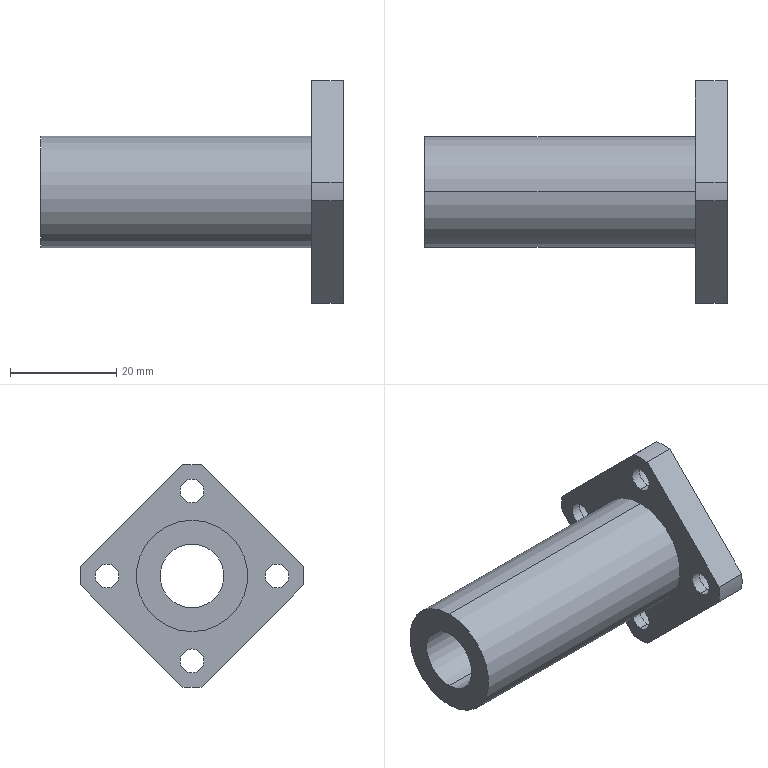Part | SolidWorks | features HoleWzd 2, ICE 2, CirPattern 1, Extrusion 1 | 1 solid | 36 faces | box 57 x 42 x 42 mm | volume 16451 mm3 | cylinder 25 | plane 11 | commonest cylinder face diameters 4.5 x8 7.5 x8 42 x5 12 x2 21 x2
STEP:
#1=CARTESIAN_POINT('',(22.5,0.,-13.75));
#2=VERTEX_POINT('',#1);
#3=CARTESIAN_POINT('',(22.5,0.,-18.25));
#4=VERTEX_POINT('',#3);
#5=CARTESIAN_POINT('',(22.5,0.,-16.));
#6=DIRECTION('',(1.,0.,0.));
#7=DIRECTION('',(0.,0.,-1.));
#8=AXIS2_PLACEMENT_3D('',#5,#6,#7);
#9=CIRCLE('',#8,2.25);
#10=EDGE_CURVE('',#2,#4,#9,.T.);
#11=ORIENTED_EDGE('',*,*,#10,.F.);
#12=CARTESIAN_POINT('',(24.4,0.,-13.75));
#13=VERTEX_POINT('',#12);
#14=CARTESIAN_POINT('',(24.4,0.,-13.75));
#15=DIRECTION('',(1.,0.,0.));
#16=VECTOR('',#15,1000.);
#17=LINE('',#14,#16);
#18=EDGE_CURVE('',#2,#13,#17,.T.);
#19=ORIENTED_EDGE('',*,*,#18,.T.);
#20=CARTESIAN_POINT('',(24.4,0.,-18.25));
#21=VERTEX_POINT('',#20);
#22=CARTESIAN_POINT('',(24.4,0.,-16.));
#23=DIRECTION('',(1.,0.,0.));
#24=DIRECTION('',(0.,0.,-1.));
#25=AXIS2_PLACEMENT_3D('',#22,#23,#24);
#26=CIRCLE('',#25,2.25);
#27=EDGE_CURVE('',#13,#21,#26,.T.);
#28=ORIENTED_EDGE('',*,*,#27,.T.);
#29=CARTESIAN_POINT('',(24.4,0.,-18.25));
#30=DIRECTION('',(1.,0.,0.));
#31=VECTOR('',#30,1000.);
#32=LINE('',#29,#31);
#33=EDGE_CURVE('',#4,#21,#32,.T.);
#34=ORIENTED_EDGE('',*,*,#33,.F.);
#35=EDGE_LOOP('',(#11,#19,#28,#34));
#36=FACE_OUTER_BOUND('',#35,.T.);
#37=CARTESIAN_POINT('',(24.4,0.,-16.));
#38=DIRECTION('',(1.,0.,0.));
#39=DIRECTION('',(0.,0.,-1.));
#40=AXIS2_PLACEMENT_3D('',#37,#38,#39);
#41=CYLINDRICAL_SURFACE('',#40,2.25);
#42=ADVANCED_FACE('',(#36),#41,.F.);
#43=CARTESIAN_POINT('',(22.5,-16.,2.25));
#44=VERTEX_POINT('',#43);
#45=CARTESIAN_POINT('',(22.5,-16.,-2.25));
#46=VERTEX_POINT('',#45);
#47=CARTESIAN_POINT('',(22.5,-16.,0.));
#48=DIRECTION('',(1.,0.,0.));
#49=DIRECTION('',(0.,0.,-1.));
#50=AXIS2_PLACEMENT_3D('',#47,#48,#49);
#51=CIRCLE('',#50,2.25);
#52=EDGE_CURVE('',#44,#46,#51,.T.);
#53=ORIENTED_EDGE('',*,*,#52,.F.);
#54=CARTESIAN_POINT('',(24.4,-16.,2.25));
#55=VERTEX_POINT('',#54);
#56=CARTESIAN_POINT('',(24.4,-16.,2.25));
#57=DIRECTION('',(1.,0.,0.));
#58=VECTOR('',#57,1000.);
#59=LINE('',#56,#58);
#60=EDGE_CURVE('',#44,#55,#59,.T.);
#61=ORIENTED_EDGE('',*,*,#60,.T.);
#62=CARTESIAN_POINT('',(24.4,-16.,-2.25));
#63=VERTEX_POINT('',#62);
#64=CARTESIAN_POINT('',(24.4,-16.,0.));
#65=DIRECTION('',(1.,0.,0.));
#66=DIRECTION('',(0.,0.,-1.));
#67=AXIS2_PLACEMENT_3D('',#64,#65,#66);
#68=CIRCLE('',#67,2.25);
#69=EDGE_CURVE('',#55,#63,#68,.T.);
#70=ORIENTED_EDGE('',*,*,#69,.T.);
#71=CARTESIAN_POINT('',(24.4,-16.,-2.25));
#72=DIRECTION('',(1.,0.,0.));
#73=VECTOR('',#72,1000.);
#74=LINE('',#71,#73);
#75=EDGE_CURVE('',#46,#63,#74,.T.);
#76=ORIENTED_EDGE('',*,*,#75,.F.);
#77=EDGE_LOOP('',(#53,#61,#70,#76));
#78=FACE_OUTER_BOUND('',#77,.T.);
#79=CARTESIAN_POINT('',(24.4,-16.,0.));
#80=DIRECTION('',(1.,0.,0.));
#81=DIRECTION('',(0.,0.,-1.));
#82=AXIS2_PLACEMENT_3D('',#79,#80,#81);
#83=CYLINDRICAL_SURFACE('',#82,2.25);
#84=ADVANCED_FACE('',(#78),#83,.F.);
#85=CARTESIAN_POINT('',(22.5,0.,18.25));
#86=VERTEX_POINT('',#85);
#87=CARTESIAN_POINT('',(22.5,0.,13.75));
#88=VERTEX_POINT('',#87);
#89=CARTESIAN_POINT('',(22.5,0.,16.));
#90=DIRECTION('',(1.,0.,0.));
#91=DIRECTION('',(0.,0.,-1.));
#92=AXIS2_PLACEMENT_3D('',#89,#90,#91);
#93=CIRCLE('',#92,2.25);
#94=EDGE_CURVE('',#86,#88,#93,.T.);
#95=ORIENTED_EDGE('',*,*,#94,.F.);
#96=CARTESIAN_POINT('',(24.4,0.,18.25));
#97=VERTEX_POINT('',#96);
#98=CARTESIAN_POINT('',(24.4,0.,18.25));
#99=DIRECTION('',(1.,0.,0.));
#100=VECTOR('',#99,1000.);
#101=LINE('',#98,#100);
#102=EDGE_CURVE('',#86,#97,#101,.T.);
#103=ORIENTED_EDGE('',*,*,#102,.T.);
#104=CARTESIAN_POINT('',(24.4,0.,13.75));
#105=VERTEX_POINT('',#104);
#106=CARTESIAN_POINT('',(24.4,0.,16.));
#107=DIRECTION('',(1.,0.,0.));
#108=DIRECTION('',(0.,0.,-1.));
#109=AXIS2_PLACEMENT_3D('',#106,#107,#108);
#110=CIRCLE('',#109,2.25);
#111=EDGE_CURVE('',#97,#105,#110,.T.);
#112=ORIENTED_EDGE('',*,*,#111,.T.);
#113=CARTESIAN_POINT('',(24.4,0.,13.75));
#114=DIRECTION('',(1.,0.,0.));
#115=VECTOR('',#114,1000.);
#116=LINE('',#113,#115);
#117=EDGE_CURVE('',#88,#105,#116,.T.);
#118=ORIENTED_EDGE('',*,*,#117,.F.);
#119=EDGE_LOOP('',(#95,#103,#112,#118));
#120=FACE_OUTER_BOUND('',#119,.T.);
#121=CARTESIAN_POINT('',(24.4,0.,16.));
#122=DIRECTION('',(1.,0.,0.));
#123=DIRECTION('',(0.,0.,-1.));
#124=AXIS2_PLACEMENT_3D('',#121,#122,#123);
#125=CYLINDRICAL_SURFACE('',#124,2.25);
#126=ADVANCED_FACE('',(#120),#125,.F.);
#127=CARTESIAN_POINT('',(24.4,0.,-12.25));
#128=VERTEX_POINT('',#127);
#129=CARTESIAN_POINT('',(24.4,0.,-19.75));
#130=VERTEX_POINT('',#129);
#131=CARTESIAN_POINT('',(24.4,0.,-16.));
#132=DIRECTION('',(1.,0.,0.));
#133=DIRECTION('',(0.,0.,-1.));
#134=AXIS2_PLACEMENT_3D('',#131,#132,#133);
#135=CIRCLE('',#134,3.75);
#136=EDGE_CURVE('',#128,#130,#135,.T.);
#137=ORIENTED_EDGE('',*,*,#136,.F.);
#138=CARTESIAN_POINT('',(28.5,0.,-12.25));
#139=VERTEX_POINT('',#138);
#140=CARTESIAN_POINT('',(28.5,0.,-12.25));
#141=DIRECTION('',(1.,0.,0.));
#142=VECTOR('',#141,1000.);
#143=LINE('',#140,#142);
#144=EDGE_CURVE('',#128,#139,#143,.T.);
#145=ORIENTED_EDGE('',*,*,#144,.T.);
#146=CARTESIAN_POINT('',(28.5,0.,-19.75));
#147=VERTEX_POINT('',#146);
#148=CARTESIAN_POINT('',(28.5,0.,-16.));
#149=DIRECTION('',(1.,0.,0.));
#150=DIRECTION('',(0.,0.,-1.));
#151=AXIS2_PLACEMENT_3D('',#148,#149,#150);
#152=CIRCLE('',#151,3.75);
#153=EDGE_CURVE('',#139,#147,#152,.T.);
#154=ORIENTED_EDGE('',*,*,#153,.T.);
#155=CARTESIAN_POINT('',(28.5,0.,-19.75));
#156=DIRECTION('',(1.,0.,0.));
#157=VECTOR('',#156,1000.);
#158=LINE('',#155,#157);
#159=EDGE_CURVE('',#130,#147,#158,.T.);
#160=ORIENTED_EDGE('',*,*,#159,.F.);
#161=EDGE_LOOP('',(#137,#145,#154,#160));
#162=FACE_OUTER_BOUND('',#161,.T.);
#163=CARTESIAN_POINT('',(28.5,0.,-16.));
#164=DIRECTION('',(1.,0.,0.));
#165=DIRECTION('',(0.,0.,-1.));
#166=AXIS2_PLACEMENT_3D('',#163,#164,#165);
#167=CYLINDRICAL_SURFACE('',#166,3.75);
#168=ADVANCED_FACE('',(#162),#167,.F.);
#169=CARTESIAN_POINT('',(24.4,-16.,3.75));
#170=VERTEX_POINT('',#169);
#171=CARTESIAN_POINT('',(24.4,-16.,-3.75));
#172=VERTEX_POINT('',#171);
#173=CARTESIAN_POINT('',(24.4,-16.,0.));
#174=DIRECTION('',(1.,0.,0.));
#175=DIRECTION('',(0.,0.,-1.));
#176=AXIS2_PLACEMENT_3D('',#173,#174,#175);
#177=CIRCLE('',#176,3.75);
#178=EDGE_CURVE('',#170,#172,#177,.T.);
#179=ORIENTED_EDGE('',*,*,#178,.F.);
#180=CARTESIAN_POINT('',(28.5,-16.,3.75));
#181=VERTEX_POINT('',#180);
#182=CARTESIAN_POINT('',(28.5,-16.,3.75));
#183=DIRECTION('',(1.,0.,0.));
#184=VECTOR('',#183,1000.);
#185=LINE('',#182,#184);
#186=EDGE_CURVE('',#170,#181,#185,.T.);
#187=ORIENTED_EDGE('',*,*,#186,.T.);
#188=CARTESIAN_POINT('',(28.5,-16.,-3.75));
#189=VERTEX_POINT('',#188);
#190=CARTESIAN_POINT('',(28.5,-16.,0.));
#191=DIRECTION('',(1.,0.,0.));
#192=DIRECTION('',(0.,0.,-1.));
#193=AXIS2_PLACEMENT_3D('',#190,#191,#192);
#194=CIRCLE('',#193,3.75);
#195=EDGE_CURVE('',#181,#189,#194,.T.);
#196=ORIENTED_EDGE('',*,*,#195,.T.);
#197=CARTESIAN_POINT('',(28.5,-16.,-3.75));
#198=DIRECTION('',(1.,0.,0.));
#199=VECTOR('',#198,1000.);
#200=LINE('',#197,#199);
#201=EDGE_CURVE('',#172,#189,#200,.T.);
#202=ORIENTED_EDGE('',*,*,#201,.F.);
#203=EDGE_LOOP('',(#179,#187,#196,#202));
#204=FACE_OUTER_BOUND('',#203,.T.);
#205=CARTESIAN_POINT('',(28.5,-16.,0.));
#206=DIRECTION('',(1.,0.,0.));
#207=DIRECTION('',(0.,0.,-1.));
#208=AXIS2_PLACEMENT_3D('',#205,#206,#207);
#209=CYLINDRICAL_SURFACE('',#208,3.75);
#210=ADVANCED_FACE('',(#204),#209,.F.);
#211=CARTESIAN_POINT('',(24.4,0.,19.75));
#212=VERTEX_POINT('',#211);
#213=CARTESIAN_POINT('',(24.4,0.,12.25));
#214=VERTEX_POINT('',#213);
#215=CARTESIAN_POINT('',(24.4,0.,16.));
#216=DIRECTION('',(1.,0.,0.));
#217=DIRECTION('',(0.,0.,-1.));
#218=AXIS2_PLACEMENT_3D('',#215,#216,#217);
#219=CIRCLE('',#218,3.75);
#220=EDGE_CURVE('',#212,#214,#219,.T.);
#221=ORIENTED_EDGE('',*,*,#220,.F.);
#222=CARTESIAN_POINT('',(28.5,0.,19.75));
#223=VERTEX_POINT('',#222);
#224=CARTESIAN_POINT('',(28.5,0.,19.75));
#225=DIRECTION('',(1.,0.,0.));
#226=VECTOR('',#225,1000.);
#227=LINE('',#224,#226);
#228=EDGE_CURVE('',#212,#223,#227,.T.);
#229=ORIENTED_EDGE('',*,*,#228,.T.);
#230=CARTESIAN_POINT('',(28.5,0.,12.25));
#231=VERTEX_POINT('',#230);
#232=CARTESIAN_POINT('',(28.5,0.,16.));
#233=DIRECTION('',(1.,0.,0.));
#234=DIRECTION('',(0.,0.,-1.));
#235=AXIS2_PLACEMENT_3D('',#232,#233,#234);
#236=CIRCLE('',#235,3.75);
#237=EDGE_CURVE('',#223,#231,#236,.T.);
#238=ORIENTED_EDGE('',*,*,#237,.T.);
#239=CARTESIAN_POINT('',(28.5,0.,12.25));
#240=DIRECTION('',(1.,0.,0.));
#241=VECTOR('',#240,1000.);
#242=LINE('',#239,#241);
#243=EDGE_CURVE('',#214,#231,#242,.T.);
#244=ORIENTED_EDGE('',*,*,#243,.F.);
#245=EDGE_LOOP('',(#221,#229,#238,#244));
#246=FACE_OUTER_BOUND('',#245,.T.);
#247=CARTESIAN_POINT('',(28.5,0.,16.));
#248=DIRECTION('',(1.,0.,0.));
#249=DIRECTION('',(0.,0.,-1.));
#250=AXIS2_PLACEMENT_3D('',#247,#248,#249);
#251=CYLINDRICAL_SURFACE('',#250,3.75);
#252=ADVANCED_FACE('',(#246),#251,.F.);
#253=CARTESIAN_POINT('',(22.5,16.,2.25));
#254=VERTEX_POINT('',#253);
#255=CARTESIAN_POINT('',(22.5,16.,-2.25));
#256=VERTEX_POINT('',#255);
#257=CARTESIAN_POINT('',(22.5,16.,0.));
#258=DIRECTION('',(1.,0.,0.));
#259=DIRECTION('',(0.,0.,-1.));
#260=AXIS2_PLACEMENT_3D('',#257,#258,#259);
#261=CIRCLE('',#260,2.25);
#262=EDGE_CURVE('',#254,#256,#261,.T.);
#263=ORIENTED_EDGE('',*,*,#262,.F.);
#264=CARTESIAN_POINT('',(24.4,16.,2.25));
#265=VERTEX_POINT('',#264);
#266=CARTESIAN_POINT('',(24.4,16.,2.25));
#267=DIRECTION('',(1.,0.,0.));
#268=VECTOR('',#267,1000.);
#269=LINE('',#266,#268);
#270=EDGE_CURVE('',#254,#265,#269,.T.);
#271=ORIENTED_EDGE('',*,*,#270,.T.);
#272=CARTESIAN_POINT('',(24.4,16.,-2.25));
#273=VERTEX_POINT('',#272);
#274=CARTESIAN_POINT('',(24.4,16.,0.));
#275=DIRECTION('',(1.,0.,0.));
#276=DIRECTION('',(0.,0.,-1.));
#277=AXIS2_PLACEMENT_3D('',#274,#275,#276);
#278=CIRCLE('',#277,2.25);
#279=EDGE_CURVE('',#265,#273,#278,.T.);
#280=ORIENTED_EDGE('',*,*,#279,.T.);
#281=CARTESIAN_POINT('',(24.4,16.,-2.25));
#282=DIRECTION('',(1.,0.,0.));
#283=VECTOR('',#282,1000.);
#284=LINE('',#281,#283);
#285=EDGE_CURVE('',#256,#273,#284,.T.);
#286=ORIENTED_EDGE('',*,*,#285,.F.);
#287=EDGE_LOOP('',(#263,#271,#280,#286));
#288=FACE_OUTER_BOUND('',#287,.T.);
#289=CARTESIAN_POINT('',(24.4,16.,0.));
#290=DIRECTION('',(1.,0.,0.));
#291=DIRECTION('',(0.,0.,-1.));
#292=AXIS2_PLACEMENT_3D('',#289,#290,#291);
#293=CYLINDRICAL_SURFACE('',#292,2.25);
#294=ADVANCED_FACE('',(#288),#293,.F.);
#295=CARTESIAN_POINT('',(24.4,16.,3.75));
#296=VERTEX_POINT('',#295);
#297=CARTESIAN_POINT('',(24.4,16.,-3.75));
#298=VERTEX_POINT('',#297);
#299=CARTESIAN_POINT('',(24.4,16.,0.));
#300=DIRECTION('',(1.,0.,0.));
#301=DIRECTION('',(0.,0.,-1.));
#302=AXIS2_PLACEMENT_3D('',#299,#300,#301);
#303=CIRCLE('',#302,3.75);
#304=EDGE_CURVE('',#296,#298,#303,.T.);
#305=ORIENTED_EDGE('',*,*,#304,.F.);
#306=CARTESIAN_POINT('',(28.5,16.,3.75));
#307=VERTEX_POINT('',#306);
#308=CARTESIAN_POINT('',(28.5,16.,3.75));
#309=DIRECTION('',(1.,0.,0.));
#310=VECTOR('',#309,1000.);
#311=LINE('',#308,#310);
#312=EDGE_CURVE('',#296,#307,#311,.T.);
#313=ORIENTED_EDGE('',*,*,#312,.T.);
#314=CARTESIAN_POINT('',(28.5,16.,-3.75));
#315=VERTEX_POINT('',#314);
#316=CARTESIAN_POINT('',(28.5,16.,0.));
#317=DIRECTION('',(1.,0.,0.));
#318=DIRECTION('',(0.,0.,-1.));
#319=AXIS2_PLACEMENT_3D('',#316,#317,#318);
#320=CIRCLE('',#319,3.75);
#321=EDGE_CURVE('',#307,#315,#320,.T.);
#322=ORIENTED_EDGE('',*,*,#321,.T.);
#323=CARTESIAN_POINT('',(28.5,16.,-3.75));
#324=DIRECTION('',(1.,0.,0.));
#325=VECTOR('',#324,1000.);
#326=LINE('',#323,#325);
#327=EDGE_CURVE('',#298,#315,#326,.T.);
#328=ORIENTED_EDGE('',*,*,#327,.F.);
#329=EDGE_LOOP('',(#305,#313,#322,#328));
#330=FACE_OUTER_BOUND('',#329,.T.);
#331=CARTESIAN_POINT('',(28.5,16.,0.));
#332=DIRECTION('',(1.,0.,0.));
#333=DIRECTION('',(0.,0.,-1.));
#334=AXIS2_PLACEMENT_3D('',#331,#332,#333);
#335=CYLINDRICAL_SURFACE('',#334,3.75);
#336=ADVANCED_FACE('',(#330),#335,.F.);
#337=CARTESIAN_POINT('',(22.5,-1.696,-20.931));
#338=VERTEX_POINT('',#337);
#339=CARTESIAN_POINT('',(22.5,0.,-21.));
#340=VERTEX_POINT('',#339);
#341=CARTESIAN_POINT('',(22.5,0.,0.));
#342=DIRECTION('',(1.,0.,0.));
#343=DIRECTION('',(0.,0.,-1.));
#344=AXIS2_PLACEMENT_3D('',#341,#342,#343);
#345=CIRCLE('',#344,21.);
#346=EDGE_CURVE('',#338,#340,#345,.T.);
#347=ORIENTED_EDGE('',*,*,#346,.T.);
#348=CARTESIAN_POINT('',(28.5,0.,-21.));
#349=VERTEX_POINT('',#348);
#350=CARTESIAN_POINT('',(22.5,0.,-21.));
#351=DIRECTION('',(1.,0.,0.));
#352=VECTOR('',#351,1000.);
#353=LINE('',#350,#352);
#354=EDGE_CURVE('',#340,#349,#353,.T.);
#355=ORIENTED_EDGE('',*,*,#354,.T.);
#356=CARTESIAN_POINT('',(28.5,-1.696,-20.931));
#357=VERTEX_POINT('',#356);
#358=CARTESIAN_POINT('',(28.5,0.,0.));
#359=DIRECTION('',(1.,0.,0.));
#360=DIRECTION('',(0.,0.,-1.));
#361=AXIS2_PLACEMENT_3D('',#358,#359,#360);
#362=CIRCLE('',#361,21.);
#363=EDGE_CURVE('',#357,#349,#362,.T.);
#364=ORIENTED_EDGE('',*,*,#363,.F.);
#365=CARTESIAN_POINT('',(22.5,-1.696,-20.931));
#366=DIRECTION('',(1.,0.,0.));
#367=VECTOR('',#366,1000.);
#368=LINE('',#365,#367);
#369=EDGE_CURVE('',#338,#357,#368,.T.);
#370=ORIENTED_EDGE('',*,*,#369,.F.);
#371=EDGE_LOOP('',(#347,#355,#364,#370));
#372=FACE_OUTER_BOUND('',#371,.T.);
#373=CARTESIAN_POINT('',(22.5,0.,0.));
#374=DIRECTION('',(1.,0.,0.));
#375=DIRECTION('',(0.,0.,-1.));
#376=AXIS2_PLACEMENT_3D('',#373,#374,#375);
#377=CYLINDRICAL_SURFACE('',#376,21.);
#378=ADVANCED_FACE('',(#372),#377,.T.);
#379=CARTESIAN_POINT('',(28.5,0.,6.));
#380=VERTEX_POINT('',#379);
#381=CARTESIAN_POINT('',(28.5,0.,-6.));
#382=VERTEX_POINT('',#381);
#383=CARTESIAN_POINT('',(28.5,0.,0.));
#384=DIRECTION('',(1.,0.,0.));
#385=DIRECTION('',(0.,0.,-1.));
#386=AXIS2_PLACEMENT_3D('',#383,#384,#385);
#387=CIRCLE('',#386,6.);
#388=EDGE_CURVE('',#380,#382,#387,.T.);
#389=ORIENTED_EDGE('',*,*,#388,.T.);
#390=CARTESIAN_POINT('',(-28.5,0.,-6.));
#391=VERTEX_POINT('',#390);
#392=CARTESIAN_POINT('',(28.5,0.,-6.));
#393=DIRECTION('',(-1.,0.,0.));
#394=VECTOR('',#393,1000.);
#395=LINE('',#392,#394);
#396=EDGE_CURVE('',#382,#391,#395,.T.);
#397=ORIENTED_EDGE('',*,*,#396,.T.);
#398=CARTESIAN_POINT('',(-28.5,0.,6.));
#399=VERTEX_POINT('',#398);
#400=CARTESIAN_POINT('',(-28.5,0.,0.));
#401=DIRECTION('',(1.,0.,0.));
#402=DIRECTION('',(0.,0.,-1.));
#403=AXIS2_PLACEMENT_3D('',#400,#401,#402);
#404=CIRCLE('',#403,6.);
#405=EDGE_CURVE('',#399,#391,#404,.T.);
#406=ORIENTED_EDGE('',*,*,#405,.F.);
#407=CARTESIAN_POINT('',(28.5,0.,6.));
#408=DIRECTION('',(-1.,0.,0.));
#409=VECTOR('',#408,1000.);
#410=LINE('',#407,#409);
#411=EDGE_CURVE('',#380,#399,#410,.T.);
#412=ORIENTED_EDGE('',*,*,#411,.F.);
#413=EDGE_LOOP('',(#389,#397,#406,#412));
#414=FACE_OUTER_BOUND('',#413,.T.);
#415=CARTESIAN_POINT('',(28.5,0.,0.));
#416=DIRECTION('',(-1.,0.,0.));
#417=DIRECTION('',(0.,0.,1.));
#418=AXIS2_PLACEMENT_3D('',#415,#416,#417);
#419=CYLINDRICAL_SURFACE('',#418,6.);
#420=ADVANCED_FACE('',(#414),#419,.F.);
#421=CARTESIAN_POINT('',(22.5,0.,-10.5));
#422=VERTEX_POINT('',#421);
#423=CARTESIAN_POINT('',(22.5,0.,10.5));
#424=VERTEX_POINT('',#423);
#425=CARTESIAN_POINT('',(22.5,0.,0.));
#426=DIRECTION('',(1.,0.,0.));
#427=DIRECTION('',(0.,0.,-1.));
#428=AXIS2_PLACEMENT_3D('',#425,#426,#427);
#429=CIRCLE('',#428,10.5);
#430=EDGE_CURVE('',#422,#424,#429,.T.);
#431=ORIENTED_EDGE('',*,*,#430,.F.);
#432=CARTESIAN_POINT('',(-28.5,0.,-10.5));
#433=VERTEX_POINT('',#432);
#434=CARTESIAN_POINT('',(28.5,0.,-10.5));
#435=DIRECTION('',(-1.,0.,0.));
#436=VECTOR('',#435,1000.);
#437=LINE('',#434,#436);
#438=EDGE_CURVE('',#422,#433,#437,.T.);
#439=ORIENTED_EDGE('',*,*,#438,.T.);
#440=CARTESIAN_POINT('',(-28.5,0.,10.5));
#441=VERTEX_POINT('',#440);
#442=CARTESIAN_POINT('',(-28.5,0.,0.));
#443=DIRECTION('',(1.,0.,0.));
#444=DIRECTION('',(0.,0.,-1.));
#445=AXIS2_PLACEMENT_3D('',#442,#443,#444);
#446=CIRCLE('',#445,10.5);
#447=EDGE_CURVE('',#433,#441,#446,.T.);
#448=ORIENTED_EDGE('',*,*,#447,.T.);
#449=CARTESIAN_POINT('',(28.5,0.,10.5));
#450=DIRECTION('',(-1.,0.,0.));
#451=VECTOR('',#450,1000.);
#452=LINE('',#449,#451);
#453=EDGE_CURVE('',#424,#441,#452,.T.);
#454=ORIENTED_EDGE('',*,*,#453,.F.);
#455=EDGE_LOOP('',(#431,#439,#448,#454));
#456=FACE_OUTER_BOUND('',#455,.T.);
#457=CARTESIAN_POINT('',(28.5,0.,0.));
#458=DIRECTION('',(-1.,0.,0.));
#459=DIRECTION('',(0.,0.,1.));
#460=AXIS2_PLACEMENT_3D('',#457,#458,#459);
#461=CYLINDRICAL_SURFACE('',#460,10.5);
#462=ADVANCED_FACE('',(#456),#461,.T.);
#463=CARTESIAN_POINT('',(28.5,-20.931,1.696));
#464=VERTEX_POINT('',#463);
#465=CARTESIAN_POINT('',(28.5,-20.931,-1.696));
#466=VERTEX_POINT('',#465);
#467=CARTESIAN_POINT('',(28.5,0.,0.));
#468=DIRECTION('',(1.,0.,0.));
#469=DIRECTION('',(0.,0.,-1.));
#470=AXIS2_PLACEMENT_3D('',#467,#468,#469);
#471=CIRCLE('',#470,21.);
#472=EDGE_CURVE('',#464,#466,#471,.T.);
#473=ORIENTED_EDGE('',*,*,#472,.F.);
#474=CARTESIAN_POINT('',(22.5,-20.931,1.696));
#475=VERTEX_POINT('',#474);
#476=CARTESIAN_POINT('',(22.5,-20.931,1.696));
#477=DIRECTION('',(1.,0.,0.));
#478=VECTOR('',#477,1000.);
#479=LINE('',#476,#478);
#480=EDGE_CURVE('',#475,#464,#479,.T.);
#481=ORIENTED_EDGE('',*,*,#480,.F.);
#482=CARTESIAN_POINT('',(22.5,-20.931,-1.696));
#483=VERTEX_POINT('',#482);
#484=CARTESIAN_POINT('',(22.5,0.,0.));
#485=DIRECTION('',(1.,0.,0.));
#486=DIRECTION('',(0.,0.,-1.));
#487=AXIS2_PLACEMENT_3D('',#484,#485,#486);
#488=CIRCLE('',#487,21.);
#489=EDGE_CURVE('',#475,#483,#488,.T.);
#490=ORIENTED_EDGE('',*,*,#489,.T.);
#491=CARTESIAN_POINT('',(22.5,-20.931,-1.696));
#492=DIRECTION('',(-1.,0.,0.));
#493=VECTOR('',#492,1000.);
#494=LINE('',#491,#493);
#495=EDGE_CURVE('',#466,#483,#494,.T.);
#496=ORIENTED_EDGE('',*,*,#495,.F.);
#497=EDGE_LOOP('',(#473,#481,#490,#496));
#498=FACE_OUTER_BOUND('',#497,.T.);
#499=CARTESIAN_POINT('',(22.5,0.,0.));
#500=DIRECTION('',(1.,0.,0.));
#501=DIRECTION('',(0.,0.,-1.));
#502=AXIS2_PLACEMENT_3D('',#499,#500,#501);
#503=CYLINDRICAL_SURFACE('',#502,21.);
#504=ADVANCED_FACE('',(#498),#503,.T.);
#505=CARTESIAN_POINT('',(22.5,1.696,20.931));
#506=VERTEX_POINT('',#505);
#507=CARTESIAN_POINT('',(22.5,-1.696,20.931));
#508=VERTEX_POINT('',#507);
#509=CARTESIAN_POINT('',(22.5,0.,0.));
#510=DIRECTION('',(1.,0.,0.));
#511=DIRECTION('',(0.,0.,-1.));
#512=AXIS2_PLACEMENT_3D('',#509,#510,#511);
#513=CIRCLE('',#512,21.);
#514=EDGE_CURVE('',#506,#508,#513,.T.);
#515=ORIENTED_EDGE('',*,*,#514,.T.);
#516=CARTESIAN_POINT('',(28.5,-1.696,20.931));
#517=VERTEX_POINT('',#516);
#518=CARTESIAN_POINT('',(22.5,-1.696,20.931));
#519=DIRECTION('',(-1.,0.,0.));
#520=VECTOR('',#519,1000.);
#521=LINE('',#518,#520);
#522=EDGE_CURVE('',#517,#508,#521,.T.);
#523=ORIENTED_EDGE('',*,*,#522,.F.);
#524=CARTESIAN_POINT('',(28.5,1.696,20.931));
#525=VERTEX_POINT('',#524);
#526=CARTESIAN_POINT('',(28.5,0.,0.));
#527=DIRECTION('',(1.,0.,0.));
#528=DIRECTION('',(0.,0.,-1.));
#529=AXIS2_PLACEMENT_3D('',#526,#527,#528);
#530=CIRCLE('',#529,21.);
#531=EDGE_CURVE('',#525,#517,#530,.T.);
#532=ORIENTED_EDGE('',*,*,#531,.F.);
#533=CARTESIAN_POINT('',(22.5,1.696,20.931));
#534=DIRECTION('',(1.,0.,0.));
#535=VECTOR('',#534,1000.);
#536=LINE('',#533,#535);
#537=EDGE_CURVE('',#506,#525,#536,.T.);
#538=ORIENTED_EDGE('',*,*,#537,.F.);
#539=EDGE_LOOP('',(#515,#523,#532,#538));
#540=FACE_OUTER_BOUND('',#539,.T.);
#541=CARTESIAN_POINT('',(22.5,0.,0.));
#542=DIRECTION('',(1.,0.,0.));
#543=DIRECTION('',(0.,0.,-1.));
#544=AXIS2_PLACEMENT_3D('',#541,#542,#543);
#545=CYLINDRICAL_SURFACE('',#544,21.);
#546=ADVANCED_FACE('',(#540),#545,.T.);
#547=CARTESIAN_POINT('',(22.5,20.931,-1.696));
#548=VERTEX_POINT('',#547);
#549=CARTESIAN_POINT('',(22.5,20.931,1.696));
#550=VERTEX_POINT('',#549);
#551=CARTESIAN_POINT('',(22.5,0.,0.));
#552=DIRECTION('',(1.,0.,0.));
#553=DIRECTION('',(0.,0.,-1.));
#554=AXIS2_PLACEMENT_3D('',#551,#552,#553);
#555=CIRCLE('',#554,21.);
#556=EDGE_CURVE('',#548,#550,#555,.T.);
#557=ORIENTED_EDGE('',*,*,#556,.T.);
#558=CARTESIAN_POINT('',(28.5,20.931,1.696));
#559=VERTEX_POINT('',#558);
#560=CARTESIAN_POINT('',(22.5,20.931,1.696));
#561=DIRECTION('',(-1.,0.,0.));
#562=VECTOR('',#561,1000.);
#563=LINE('',#560,#562);
#564=EDGE_CURVE('',#559,#550,#563,.T.);
#565=ORIENTED_EDGE('',*,*,#564,.F.);
#566=CARTESIAN_POINT('',(28.5,20.931,-1.696));
#567=VERTEX_POINT('',#566);
#568=CARTESIAN_POINT('',(28.5,0.,0.));
#569=DIRECTION('',(1.,0.,0.));
#570=DIRECTION('',(0.,0.,-1.));
#571=AXIS2_PLACEMENT_3D('',#568,#569,#570);
#572=CIRCLE('',#571,21.);
#573=EDGE_CURVE('',#567,#559,#572,.T.);
#574=ORIENTED_EDGE('',*,*,#573,.F.);
#575=CARTESIAN_POINT('',(22.5,20.931,-1.696));
#576=DIRECTION('',(1.,0.,0.));
#577=VECTOR('',#576,1000.);
#578=LINE('',#575,#577);
#579=EDGE_CURVE('',#548,#567,#578,.T.);
#580=ORIENTED_EDGE('',*,*,#579,.F.);
#581=EDGE_LOOP('',(#557,#565,#574,#580));
#582=FACE_OUTER_BOUND('',#581,.T.);
#583=CARTESIAN_POINT('',(22.5,0.,0.));
#584=DIRECTION('',(1.,0.,0.));
#585=DIRECTION('',(0.,0.,-1.));
#586=AXIS2_PLACEMENT_3D('',#583,#584,#585);
#587=CYLINDRICAL_SURFACE('',#586,21.);
#588=ADVANCED_FACE('',(#582),#587,.T.);
#589=CARTESIAN_POINT('',(24.4,0.,-16.));
#590=DIRECTION('',(1.,0.,0.));
#591=DIRECTION('',(0.,0.,-1.));
#592=AXIS2_PLACEMENT_3D('',#589,#590,#591);
#593=CIRCLE('',#592,3.75);
#594=EDGE_CURVE('',#130,#128,#593,.T.);
#595=ORIENTED_EDGE('',*,*,#594,.T.);
#596=ORIENTED_EDGE('',*,*,#136,.T.);
#597=EDGE_LOOP('',(#595,#596));
#598=FACE_OUTER_BOUND('',#597,.T.);
#599=CARTESIAN_POINT('',(24.4,0.,-16.));
#600=DIRECTION('',(1.,0.,0.));
#601=DIRECTION('',(0.,0.,-1.));
#602=AXIS2_PLACEMENT_3D('',#599,#600,#601);
#603=CIRCLE('',#602,2.25);
#604=EDGE_CURVE('',#21,#13,#603,.T.);
#605=ORIENTED_EDGE('',*,*,#604,.F.);
#606=ORIENTED_EDGE('',*,*,#27,.F.);
#607=EDGE_LOOP('',(#605,#606));
#608=FACE_BOUND('',#607,.T.);
#609=CARTESIAN_POINT('',(24.4,0.,-16.));
#610=DIRECTION('',(-1.,0.,0.));
#611=DIRECTION('',(0.,0.,1.));
#612=AXIS2_PLACEMENT_3D('',#609,#610,#611);
#613=PLANE('',#612);
#614=ADVANCED_FACE('',(#598,#608),#613,.F.);
#615=CARTESIAN_POINT('',(24.4,-16.,0.));
#616=DIRECTION('',(1.,0.,0.));
#617=DIRECTION('',(0.,0.,-1.));
#618=AXIS2_PLACEMENT_3D('',#615,#616,#617);
#619=CIRCLE('',#618,3.75);
#620=EDGE_CURVE('',#172,#170,#619,.T.);
#621=ORIENTED_EDGE('',*,*,#620,.T.);
#622=ORIENTED_EDGE('',*,*,#178,.T.);
#623=EDGE_LOOP('',(#621,#622));
#624=FACE_OUTER_BOUND('',#623,.T.);
#625=CARTESIAN_POINT('',(24.4,-16.,0.));
#626=DIRECTION('',(1.,0.,0.));
#627=DIRECTION('',(0.,0.,-1.));
#628=AXIS2_PLACEMENT_3D('',#625,#626,#627);
#629=CIRCLE('',#628,2.25);
#630=EDGE_CURVE('',#63,#55,#629,.T.);
#631=ORIENTED_EDGE('',*,*,#630,.F.);
#632=ORIENTED_EDGE('',*,*,#69,.F.);
#633=EDGE_LOOP('',(#631,#632));
#634=FACE_BOUND('',#633,.T.);
#635=CARTESIAN_POINT('',(24.4,-16.,0.));
#636=DIRECTION('',(-1.,0.,0.));
#637=DIRECTION('',(0.,0.,1.));
#638=AXIS2_PLACEMENT_3D('',#635,#636,#637);
#639=PLANE('',#638);
#640=ADVANCED_FACE('',(#624,#634),#639,.F.);
#641=CARTESIAN_POINT('',(24.4,0.,16.));
#642=DIRECTION('',(1.,0.,0.));
#643=DIRECTION('',(0.,0.,-1.));
#644=AXIS2_PLACEMENT_3D('',#641,#642,#643);
#645=CIRCLE('',#644,3.75);
#646=EDGE_CURVE('',#214,#212,#645,.T.);
#647=ORIENTED_EDGE('',*,*,#646,.T.);
#648=ORIENTED_EDGE('',*,*,#220,.T.);
#649=EDGE_LOOP('',(#647,#648));
#650=FACE_OUTER_BOUND('',#649,.T.);
#651=CARTESIAN_POINT('',(24.4,0.,16.));
#652=DIRECTION('',(1.,0.,0.));
#653=DIRECTION('',(0.,0.,-1.));
#654=AXIS2_PLACEMENT_3D('',#651,#652,#653);
#655=CIRCLE('',#654,2.25);
#656=EDGE_CURVE('',#105,#97,#655,.T.);
#657=ORIENTED_EDGE('',*,*,#656,.F.);
#658=ORIENTED_EDGE('',*,*,#111,.F.);
#659=EDGE_LOOP('',(#657,#658));
#660=FACE_BOUND('',#659,.T.);
#661=CARTESIAN_POINT('',(24.4,0.,16.));
#662=DIRECTION('',(-1.,0.,0.));
#663=DIRECTION('',(0.,0.,1.));
#664=AXIS2_PLACEMENT_3D('',#661,#662,#663);
#665=PLANE('',#664);
#666=ADVANCED_FACE('',(#650,#660),#665,.F.);
#667=CARTESIAN_POINT('',(24.4,16.,0.));
#668=DIRECTION('',(1.,0.,0.));
#669=DIRECTION('',(0.,0.,-1.));
#670=AXIS2_PLACEMENT_3D('',#667,#668,#669);
#671=CIRCLE('',#670,3.75);
#672=EDGE_CURVE('',#298,#296,#671,.T.);
#673=ORIENTED_EDGE('',*,*,#672,.T.);
#674=ORIENTED_EDGE('',*,*,#304,.T.);
#675=EDGE_LOOP('',(#673,#674));
#676=FACE_OUTER_BOUND('',#675,.T.);
#677=CARTESIAN_POINT('',(24.4,16.,0.));
#678=DIRECTION('',(1.,0.,0.));
#679=DIRECTION('',(0.,0.,-1.));
#680=AXIS2_PLACEMENT_3D('',#677,#678,#679);
#681=CIRCLE('',#680,2.25);
#682=EDGE_CURVE('',#273,#265,#681,.T.);
#683=ORIENTED_EDGE('',*,*,#682,.F.);
#684=ORIENTED_EDGE('',*,*,#279,.F.);
#685=EDGE_LOOP('',(#683,#684));
#686=FACE_BOUND('',#685,.T.);
#687=CARTESIAN_POINT('',(24.4,16.,0.));
#688=DIRECTION('',(-1.,0.,0.));
#689=DIRECTION('',(0.,0.,1.));
#690=AXIS2_PLACEMENT_3D('',#687,#688,#689);
#691=PLANE('',#690);
#692=ADVANCED_FACE('',(#676,#686),#691,.F.);
#693=ORIENTED_EDGE('',*,*,#438,.F.);
#694=CARTESIAN_POINT('',(22.5,0.,0.));
#695=DIRECTION('',(1.,0.,0.));
#696=DIRECTION('',(0.,0.,-1.));
#697=AXIS2_PLACEMENT_3D('',#694,#695,#696);
#698=CIRCLE('',#697,10.5);
#699=EDGE_CURVE('',#424,#422,#698,.T.);
#700=ORIENTED_EDGE('',*,*,#699,.F.);
#701=ORIENTED_EDGE('',*,*,#453,.T.);
#702=CARTESIAN_POINT('',(-28.5,0.,0.));
#703=DIRECTION('',(1.,0.,0.));
#704=DIRECTION('',(0.,0.,-1.));
#705=AXIS2_PLACEMENT_3D('',#702,#703,#704);
#706=CIRCLE('',#705,10.5);
#707=EDGE_CURVE('',#441,#433,#706,.T.);
#708=ORIENTED_EDGE('',*,*,#707,.T.);
#709=EDGE_LOOP('',(#693,#700,#701,#708));
#710=FACE_OUTER_BOUND('',#709,.T.);
#711=CARTESIAN_POINT('',(28.5,0.,0.));
#712=DIRECTION('',(-1.,0.,0.));
#713=DIRECTION('',(0.,0.,1.));
#714=AXIS2_PLACEMENT_3D('',#711,#712,#713);
#715=CYLINDRICAL_SURFACE('',#714,10.5);
#716=ADVANCED_FACE('',(#710),#715,.T.);
#717=CARTESIAN_POINT('',(28.5,0.,-16.));
#718=DIRECTION('',(1.,0.,0.));
#719=DIRECTION('',(0.,0.,-1.));
#720=AXIS2_PLACEMENT_3D('',#717,#718,#719);
#721=CIRCLE('',#720,3.75);
#722=EDGE_CURVE('',#147,#139,#721,.T.);
#723=ORIENTED_EDGE('',*,*,#722,.F.);
#724=ORIENTED_EDGE('',*,*,#153,.F.);
#725=EDGE_LOOP('',(#723,#724));
#726=FACE_BOUND('',#725,.T.);
#727=CARTESIAN_POINT('',(28.5,-16.,0.));
#728=DIRECTION('',(1.,0.,0.));
#729=DIRECTION('',(0.,0.,-1.));
#730=AXIS2_PLACEMENT_3D('',#727,#728,#729);
#731=CIRCLE('',#730,3.75);
#732=EDGE_CURVE('',#189,#181,#731,.T.);
#733=ORIENTED_EDGE('',*,*,#732,.F.);
#734=ORIENTED_EDGE('',*,*,#195,.F.);
#735=EDGE_LOOP('',(#733,#734));
#736=FACE_BOUND('',#735,.T.);
#737=CARTESIAN_POINT('',(28.5,0.,16.));
#738=DIRECTION('',(1.,0.,0.));
#739=DIRECTION('',(0.,0.,-1.));
#740=AXIS2_PLACEMENT_3D('',#737,#738,#739);
#741=CIRCLE('',#740,3.75);
#742=EDGE_CURVE('',#231,#223,#741,.T.);
#743=ORIENTED_EDGE('',*,*,#742,.F.);
#744=ORIENTED_EDGE('',*,*,#237,.F.);
#745=EDGE_LOOP('',(#743,#744));
#746=FACE_BOUND('',#745,.T.);
#747=CARTESIAN_POINT('',(28.5,16.,0.));
#748=DIRECTION('',(1.,0.,0.));
#749=DIRECTION('',(0.,0.,-1.));
#750=AXIS2_PLACEMENT_3D('',#747,#748,#749);
#751=CIRCLE('',#750,3.75);
#752=EDGE_CURVE('',#315,#307,#751,.T.);
#753=ORIENTED_EDGE('',*,*,#752,.F.);
#754=ORIENTED_EDGE('',*,*,#321,.F.);
#755=EDGE_LOOP('',(#753,#754));
#756=FACE_BOUND('',#755,.T.);
#757=ORIENTED_EDGE('',*,*,#388,.F.);
#758=CARTESIAN_POINT('',(28.5,0.,0.));
#759=DIRECTION('',(1.,0.,0.));
#760=DIRECTION('',(0.,0.,-1.));
#761=AXIS2_PLACEMENT_3D('',#758,#759,#760);
#762=CIRCLE('',#761,6.);
#763=EDGE_CURVE('',#382,#380,#762,.T.);
#764=ORIENTED_EDGE('',*,*,#763,.F.);
#765=EDGE_LOOP('',(#757,#764));
#766=FACE_BOUND('',#765,.T.);
#767=ORIENTED_EDGE('',*,*,#531,.T.);
#768=CARTESIAN_POINT('',(28.5,0.,22.627));
#769=DIRECTION('',(0.,-0.7071,-0.7071));
#770=VECTOR('',#769,1000.);
#771=LINE('',#768,#770);
#772=EDGE_CURVE('',#517,#464,#771,.T.);
#773=ORIENTED_EDGE('',*,*,#772,.T.);
#774=ORIENTED_EDGE('',*,*,#472,.T.);
#775=CARTESIAN_POINT('',(28.5,-22.627,0.));
#776=DIRECTION('',(0.,0.7071,-0.7071));
#777=VECTOR('',#776,1000.);
#778=LINE('',#775,#777);
#779=EDGE_CURVE('',#466,#357,#778,.T.);
#780=ORIENTED_EDGE('',*,*,#779,.T.);
#781=ORIENTED_EDGE('',*,*,#363,.T.);
#782=CARTESIAN_POINT('',(28.5,1.696,-20.931));
#783=VERTEX_POINT('',#782);
#784=CARTESIAN_POINT('',(28.5,0.,0.));
#785=DIRECTION('',(1.,0.,0.));
#786=DIRECTION('',(0.,0.,-1.));
#787=AXIS2_PLACEMENT_3D('',#784,#785,#786);
#788=CIRCLE('',#787,21.);
#789=EDGE_CURVE('',#349,#783,#788,.T.);
#790=ORIENTED_EDGE('',*,*,#789,.T.);
#791=CARTESIAN_POINT('',(28.5,0.,-22.627));
#792=DIRECTION('',(0.,0.7071,0.7071));
#793=VECTOR('',#792,1000.);
#794=LINE('',#791,#793);
#795=EDGE_CURVE('',#783,#567,#794,.T.);
#796=ORIENTED_EDGE('',*,*,#795,.T.);
#797=ORIENTED_EDGE('',*,*,#573,.T.);
#798=CARTESIAN_POINT('',(28.5,22.627,0.));
#799=DIRECTION('',(0.,-0.7071,0.7071));
#800=VECTOR('',#799,1000.);
#801=LINE('',#798,#800);
#802=EDGE_CURVE('',#559,#525,#801,.T.);
#803=ORIENTED_EDGE('',*,*,#802,.T.);
#804=EDGE_LOOP('',(#767,#773,#774,#780,#781,#790,#796,#797,#803));
#805=FACE_OUTER_BOUND('',#804,.T.);
#806=CARTESIAN_POINT('',(28.5,0.,0.));
#807=DIRECTION('',(1.,0.,0.));
#808=DIRECTION('',(0.,0.,-1.));
#809=AXIS2_PLACEMENT_3D('',#806,#807,#808);
#810=PLANE('',#809);
#811=ADVANCED_FACE('',(#726,#736,#746,#756,#766,#805),#810,.T.);
#812=ORIENTED_EDGE('',*,*,#707,.F.);
#813=ORIENTED_EDGE('',*,*,#447,.F.);
#814=EDGE_LOOP('',(#812,#813));
#815=FACE_OUTER_BOUND('',#814,.T.);
#816=ORIENTED_EDGE('',*,*,#405,.T.);
#817=CARTESIAN_POINT('',(-28.5,0.,0.));
#818=DIRECTION('',(1.,0.,0.));
#819=DIRECTION('',(0.,0.,-1.));
#820=AXIS2_PLACEMENT_3D('',#817,#818,#819);
#821=CIRCLE('',#820,6.);
#822=EDGE_CURVE('',#391,#399,#821,.T.);
#823=ORIENTED_EDGE('',*,*,#822,.T.);
#824=EDGE_LOOP('',(#816,#823));
#825=FACE_BOUND('',#824,.T.);
#826=CARTESIAN_POINT('',(-28.5,0.,0.));
#827=DIRECTION('',(1.,0.,0.));
#828=DIRECTION('',(0.,0.,-1.));
#829=AXIS2_PLACEMENT_3D('',#826,#827,#828);
#830=PLANE('',#829);
#831=ADVANCED_FACE('',(#815,#825),#830,.F.);
#832=ORIENTED_EDGE('',*,*,#396,.F.);
#833=ORIENTED_EDGE('',*,*,#763,.T.);
#834=ORIENTED_EDGE('',*,*,#411,.T.);
#835=ORIENTED_EDGE('',*,*,#822,.F.);
#836=EDGE_LOOP('',(#832,#833,#834,#835));
#837=FACE_OUTER_BOUND('',#836,.T.);
#838=CARTESIAN_POINT('',(28.5,0.,0.));
#839=DIRECTION('',(-1.,0.,0.));
#840=DIRECTION('',(0.,0.,1.));
#841=AXIS2_PLACEMENT_3D('',#838,#839,#840);
#842=CYLINDRICAL_SURFACE('',#841,6.);
#843=ADVANCED_FACE('',(#837),#842,.F.);
#844=CARTESIAN_POINT('',(22.5,0.,22.627));
#845=DIRECTION('',(0.,0.7071,0.7071));
#846=VECTOR('',#845,1000.);
#847=LINE('',#844,#846);
#848=EDGE_CURVE('',#475,#508,#847,.T.);
#849=ORIENTED_EDGE('',*,*,#848,.T.);
#850=ORIENTED_EDGE('',*,*,#514,.F.);
#851=CARTESIAN_POINT('',(22.5,22.627,0.));
#852=DIRECTION('',(0.,0.7071,-0.7071));
#853=VECTOR('',#852,1000.);
#854=LINE('',#851,#853);
#855=EDGE_CURVE('',#506,#550,#854,.T.);
#856=ORIENTED_EDGE('',*,*,#855,.T.);
#857=ORIENTED_EDGE('',*,*,#556,.F.);
#858=CARTESIAN_POINT('',(22.5,1.696,-20.931));
#859=VERTEX_POINT('',#858);
#860=CARTESIAN_POINT('',(22.5,0.,-22.627));
#861=DIRECTION('',(0.,-0.7071,-0.7071));
#862=VECTOR('',#861,1000.);
#863=LINE('',#860,#862);
#864=EDGE_CURVE('',#548,#859,#863,.T.);
#865=ORIENTED_EDGE('',*,*,#864,.T.);
#866=CARTESIAN_POINT('',(22.5,0.,0.));
#867=DIRECTION('',(1.,0.,0.));
#868=DIRECTION('',(0.,0.,-1.));
#869=AXIS2_PLACEMENT_3D('',#866,#867,#868);
#870=CIRCLE('',#869,21.);
#871=EDGE_CURVE('',#340,#859,#870,.T.);
#872=ORIENTED_EDGE('',*,*,#871,.F.);
#873=ORIENTED_EDGE('',*,*,#346,.F.);
#874=CARTESIAN_POINT('',(22.5,-22.627,0.));
#875=DIRECTION('',(0.,-0.7071,0.7071));
#876=VECTOR('',#875,1000.);
#877=LINE('',#874,#876);
#878=EDGE_CURVE('',#338,#483,#877,.T.);
#879=ORIENTED_EDGE('',*,*,#878,.T.);
#880=ORIENTED_EDGE('',*,*,#489,.F.);
#881=EDGE_LOOP('',(#849,#850,#856,#857,#865,#872,#873,#879,#880));
#882=FACE_OUTER_BOUND('',#881,.T.);
#883=CARTESIAN_POINT('',(22.5,0.,-16.));
#884=DIRECTION('',(1.,0.,0.));
#885=DIRECTION('',(0.,0.,-1.));
#886=AXIS2_PLACEMENT_3D('',#883,#884,#885);
#887=CIRCLE('',#886,2.25);
#888=EDGE_CURVE('',#4,#2,#887,.T.);
#889=ORIENTED_EDGE('',*,*,#888,.T.);
#890=ORIENTED_EDGE('',*,*,#10,.T.);
#891=EDGE_LOOP('',(#889,#890));
#892=FACE_BOUND('',#891,.T.);
#893=CARTESIAN_POINT('',(22.5,-16.,0.));
#894=DIRECTION('',(1.,0.,0.));
#895=DIRECTION('',(0.,0.,-1.));
#896=AXIS2_PLACEMENT_3D('',#893,#894,#895);
#897=CIRCLE('',#896,2.25);
#898=EDGE_CURVE('',#46,#44,#897,.T.);
#899=ORIENTED_EDGE('',*,*,#898,.T.);
#900=ORIENTED_EDGE('',*,*,#52,.T.);
#901=EDGE_LOOP('',(#899,#900));
#902=FACE_BOUND('',#901,.T.);
#903=CARTESIAN_POINT('',(22.5,0.,16.));
#904=DIRECTION('',(1.,0.,0.));
#905=DIRECTION('',(0.,0.,-1.));
#906=AXIS2_PLACEMENT_3D('',#903,#904,#905);
#907=CIRCLE('',#906,2.25);
#908=EDGE_CURVE('',#88,#86,#907,.T.);
#909=ORIENTED_EDGE('',*,*,#908,.T.);
#910=ORIENTED_EDGE('',*,*,#94,.T.);
#911=EDGE_LOOP('',(#909,#910));
#912=FACE_BOUND('',#911,.T.);
#913=CARTESIAN_POINT('',(22.5,16.,0.));
#914=DIRECTION('',(1.,0.,0.));
#915=DIRECTION('',(0.,0.,-1.));
#916=AXIS2_PLACEMENT_3D('',#913,#914,#915);
#917=CIRCLE('',#916,2.25);
#918=EDGE_CURVE('',#256,#254,#917,.T.);
#919=ORIENTED_EDGE('',*,*,#918,.T.);
#920=ORIENTED_EDGE('',*,*,#262,.T.);
#921=EDGE_LOOP('',(#919,#920));
#922=FACE_BOUND('',#921,.T.);
#923=ORIENTED_EDGE('',*,*,#699,.T.);
#924=ORIENTED_EDGE('',*,*,#430,.T.);
#925=EDGE_LOOP('',(#923,#924));
#926=FACE_BOUND('',#925,.T.);
#927=CARTESIAN_POINT('',(22.5,0.,0.));
#928=DIRECTION('',(1.,0.,0.));
#929=DIRECTION('',(0.,0.,-1.));
#930=AXIS2_PLACEMENT_3D('',#927,#928,#929);
#931=PLANE('',#930);
#932=ADVANCED_FACE('',(#882,#892,#902,#912,#922,#926),#931,.F.);
#933=ORIENTED_EDGE('',*,*,#354,.F.);
#934=ORIENTED_EDGE('',*,*,#871,.T.);
#935=CARTESIAN_POINT('',(22.5,1.696,-20.931));
#936=DIRECTION('',(-1.,0.,0.));
#937=VECTOR('',#936,1000.);
#938=LINE('',#935,#937);
#939=EDGE_CURVE('',#783,#859,#938,.T.);
#940=ORIENTED_EDGE('',*,*,#939,.F.);
#941=ORIENTED_EDGE('',*,*,#789,.F.);
#942=EDGE_LOOP('',(#933,#934,#940,#941));
#943=FACE_OUTER_BOUND('',#942,.T.);
#944=CARTESIAN_POINT('',(22.5,0.,0.));
#945=DIRECTION('',(1.,0.,0.));
#946=DIRECTION('',(0.,0.,-1.));
#947=AXIS2_PLACEMENT_3D('',#944,#945,#946);
#948=CYLINDRICAL_SURFACE('',#947,21.);
#949=ADVANCED_FACE('',(#943),#948,.T.);
#950=ORIENTED_EDGE('',*,*,#312,.F.);
#951=ORIENTED_EDGE('',*,*,#672,.F.);
#952=ORIENTED_EDGE('',*,*,#327,.T.);
#953=ORIENTED_EDGE('',*,*,#752,.T.);
#954=EDGE_LOOP('',(#950,#951,#952,#953));
#955=FACE_OUTER_BOUND('',#954,.T.);
#956=CARTESIAN_POINT('',(28.5,16.,0.));
#957=DIRECTION('',(1.,0.,0.));
#958=DIRECTION('',(0.,0.,-1.));
#959=AXIS2_PLACEMENT_3D('',#956,#957,#958);
#960=CYLINDRICAL_SURFACE('',#959,3.75);
#961=ADVANCED_FACE('',(#955),#960,.F.);
#962=ORIENTED_EDGE('',*,*,#270,.F.);
#963=ORIENTED_EDGE('',*,*,#918,.F.);
#964=ORIENTED_EDGE('',*,*,#285,.T.);
#965=ORIENTED_EDGE('',*,*,#682,.T.);
#966=EDGE_LOOP('',(#962,#963,#964,#965));
#967=FACE_OUTER_BOUND('',#966,.T.);
#968=CARTESIAN_POINT('',(24.4,16.,0.));
#969=DIRECTION('',(1.,0.,0.));
#970=DIRECTION('',(0.,0.,-1.));
#971=AXIS2_PLACEMENT_3D('',#968,#969,#970);
#972=CYLINDRICAL_SURFACE('',#971,2.25);
#973=ADVANCED_FACE('',(#967),#972,.F.);
#974=ORIENTED_EDGE('',*,*,#228,.F.);
#975=ORIENTED_EDGE('',*,*,#646,.F.);
#976=ORIENTED_EDGE('',*,*,#243,.T.);
#977=ORIENTED_EDGE('',*,*,#742,.T.);
#978=EDGE_LOOP('',(#974,#975,#976,#977));
#979=FACE_OUTER_BOUND('',#978,.T.);
#980=CARTESIAN_POINT('',(28.5,0.,16.));
#981=DIRECTION('',(1.,0.,0.));
#982=DIRECTION('',(0.,0.,-1.));
#983=AXIS2_PLACEMENT_3D('',#980,#981,#982);
#984=CYLINDRICAL_SURFACE('',#983,3.75);
#985=ADVANCED_FACE('',(#979),#984,.F.);
#986=ORIENTED_EDGE('',*,*,#186,.F.);
#987=ORIENTED_EDGE('',*,*,#620,.F.);
#988=ORIENTED_EDGE('',*,*,#201,.T.);
#989=ORIENTED_EDGE('',*,*,#732,.T.);
#990=EDGE_LOOP('',(#986,#987,#988,#989));
#991=FACE_OUTER_BOUND('',#990,.T.);
#992=CARTESIAN_POINT('',(28.5,-16.,0.));
#993=DIRECTION('',(1.,0.,0.));
#994=DIRECTION('',(0.,0.,-1.));
#995=AXIS2_PLACEMENT_3D('',#992,#993,#994);
#996=CYLINDRICAL_SURFACE('',#995,3.75);
#997=ADVANCED_FACE('',(#991),#996,.F.);
#998=ORIENTED_EDGE('',*,*,#144,.F.);
#999=ORIENTED_EDGE('',*,*,#594,.F.);
#1000=ORIENTED_EDGE('',*,*,#159,.T.);
#1001=ORIENTED_EDGE('',*,*,#722,.T.);
#1002=EDGE_LOOP('',(#998,#999,#1000,#1001));
#1003=FACE_OUTER_BOUND('',#1002,.T.);
#1004=CARTESIAN_POINT('',(28.5,0.,-16.));
#1005=DIRECTION('',(1.,0.,0.));
#1006=DIRECTION('',(0.,0.,-1.));
#1007=AXIS2_PLACEMENT_3D('',#1004,#1005,#1006);
#1008=CYLINDRICAL_SURFACE('',#1007,3.75);
#1009=ADVANCED_FACE('',(#1003),#1008,.F.);
#1010=ORIENTED_EDGE('',*,*,#102,.F.);
#1011=ORIENTED_EDGE('',*,*,#908,.F.);
#1012=ORIENTED_EDGE('',*,*,#117,.T.);
#1013=ORIENTED_EDGE('',*,*,#656,.T.);
#1014=EDGE_LOOP('',(#1010,#1011,#1012,#1013));
#1015=FACE_OUTER_BOUND('',#1014,.T.);
#1016=CARTESIAN_POINT('',(24.4,0.,16.));
#1017=DIRECTION('',(1.,0.,0.));
#1018=DIRECTION('',(0.,0.,-1.));
#1019=AXIS2_PLACEMENT_3D('',#1016,#1017,#1018);
#1020=CYLINDRICAL_SURFACE('',#1019,2.25);
#1021=ADVANCED_FACE('',(#1015),#1020,.F.);
#1022=ORIENTED_EDGE('',*,*,#60,.F.);
#1023=ORIENTED_EDGE('',*,*,#898,.F.);
#1024=ORIENTED_EDGE('',*,*,#75,.T.);
#1025=ORIENTED_EDGE('',*,*,#630,.T.);
#1026=EDGE_LOOP('',(#1022,#1023,#1024,#1025));
#1027=FACE_OUTER_BOUND('',#1026,.T.);
#1028=CARTESIAN_POINT('',(24.4,-16.,0.));
#1029=DIRECTION('',(1.,0.,0.));
#1030=DIRECTION('',(0.,0.,-1.));
#1031=AXIS2_PLACEMENT_3D('',#1028,#1029,#1030);
#1032=CYLINDRICAL_SURFACE('',#1031,2.25);
#1033=ADVANCED_FACE('',(#1027),#1032,.F.);
#1034=ORIENTED_EDGE('',*,*,#18,.F.);
#1035=ORIENTED_EDGE('',*,*,#888,.F.);
#1036=ORIENTED_EDGE('',*,*,#33,.T.);
#1037=ORIENTED_EDGE('',*,*,#604,.T.);
#1038=EDGE_LOOP('',(#1034,#1035,#1036,#1037));
#1039=FACE_OUTER_BOUND('',#1038,.T.);
#1040=CARTESIAN_POINT('',(24.4,0.,-16.));
#1041=DIRECTION('',(1.,0.,0.));
#1042=DIRECTION('',(0.,0.,-1.));
#1043=AXIS2_PLACEMENT_3D('',#1040,#1041,#1042);
#1044=CYLINDRICAL_SURFACE('',#1043,2.25);
#1045=ADVANCED_FACE('',(#1039),#1044,.F.);
#1046=ORIENTED_EDGE('',*,*,#878,.F.);
#1047=ORIENTED_EDGE('',*,*,#369,.T.);
#1048=ORIENTED_EDGE('',*,*,#779,.F.);
#1049=ORIENTED_EDGE('',*,*,#495,.T.);
#1050=EDGE_LOOP('',(#1046,#1047,#1048,#1049));
#1051=FACE_OUTER_BOUND('',#1050,.T.);
#1052=CARTESIAN_POINT('',(-28.501,-22.627,0.));
#1053=DIRECTION('',(0.,-0.7071,-0.7071));
#1054=DIRECTION('',(0.,0.7071,-0.7071));
#1055=AXIS2_PLACEMENT_3D('',#1052,#1053,#1054);
#1056=PLANE('',#1055);
#1057=ADVANCED_FACE('',(#1051),#1056,.T.);
#1058=ORIENTED_EDGE('',*,*,#864,.F.);
#1059=ORIENTED_EDGE('',*,*,#579,.T.);
#1060=ORIENTED_EDGE('',*,*,#795,.F.);
#1061=ORIENTED_EDGE('',*,*,#939,.T.);
#1062=EDGE_LOOP('',(#1058,#1059,#1060,#1061));
#1063=FACE_OUTER_BOUND('',#1062,.T.);
#1064=CARTESIAN_POINT('',(-28.501,0.,-22.627));
#1065=DIRECTION('',(0.,0.7071,-0.7071));
#1066=DIRECTION('',(0.,0.7071,0.7071));
#1067=AXIS2_PLACEMENT_3D('',#1064,#1065,#1066);
#1068=PLANE('',#1067);
#1069=ADVANCED_FACE('',(#1063),#1068,.T.);
#1070=ORIENTED_EDGE('',*,*,#855,.F.);
#1071=ORIENTED_EDGE('',*,*,#537,.T.);
#1072=ORIENTED_EDGE('',*,*,#802,.F.);
#1073=ORIENTED_EDGE('',*,*,#564,.T.);
#1074=EDGE_LOOP('',(#1070,#1071,#1072,#1073));
#1075=FACE_OUTER_BOUND('',#1074,.T.);
#1076=CARTESIAN_POINT('',(-28.501,22.627,0.));
#1077=DIRECTION('',(0.,0.7071,0.7071));
#1078=DIRECTION('',(0.,-0.7071,0.7071));
#1079=AXIS2_PLACEMENT_3D('',#1076,#1077,#1078);
#1080=PLANE('',#1079);
#1081=ADVANCED_FACE('',(#1075),#1080,.T.);
#1082=ORIENTED_EDGE('',*,*,#848,.F.);
#1083=ORIENTED_EDGE('',*,*,#480,.T.);
#1084=ORIENTED_EDGE('',*,*,#772,.F.);
#1085=ORIENTED_EDGE('',*,*,#522,.T.);
#1086=EDGE_LOOP('',(#1082,#1083,#1084,#1085));
#1087=FACE_OUTER_BOUND('',#1086,.T.);
#1088=CARTESIAN_POINT('',(-28.501,0.,22.627));
#1089=DIRECTION('',(0.,-0.7071,0.7071));
#1090=DIRECTION('',(0.,-0.7071,-0.7071));
#1091=AXIS2_PLACEMENT_3D('',#1088,#1089,#1090);
#1092=PLANE('',#1091);
#1093=ADVANCED_FACE('',(#1087),#1092,.T.);
#1094=CLOSED_SHELL('',(#42,#84,#126,#168,#210,#252,#294,#336,#378,#420,#462,#504,#546,#588,#614,#640,#666,#692,#716,#811,#831,#843,#932,#949,#961,#973,#985,#997,#1009,#1021,#1033,#1045,#1057,#1069,#1081,#1093));
#1095=MANIFOLD_SOLID_BREP('',#1094);
#1096=CARTESIAN_POINT('',(0.,0.,0.));
#1097=DIRECTION('',(0.,0.,1.));
#1098=DIRECTION('',(1.,0.,0.));
#1099=AXIS2_PLACEMENT_3D('',#1096,#1097,#1098);
#1100=(LENGTH_UNIT()NAMED_UNIT(*)SI_UNIT(.MILLI.,.METRE.));
#1101=UNCERTAINTY_MEASURE_WITH_UNIT(LENGTH_MEASURE(0.00001),#1100,'','');
#1102=(NAMED_UNIT(*)PLANE_ANGLE_UNIT()SI_UNIT($,.RADIAN.));
#1103=(NAMED_UNIT(*)SI_UNIT($,.STERADIAN.)SOLID_ANGLE_UNIT());
#1104=(GEOMETRIC_REPRESENTATION_CONTEXT(3)GLOBAL_UNCERTAINTY_ASSIGNED_CONTEXT((#1101))GLOBAL_UNIT_ASSIGNED_CONTEXT((#1100,#1102,#1103))REPRESENTATION_CONTEXT('',''));
#1105=ADVANCED_BREP_SHAPE_REPRESENTATION('',(#1095,#1099),#1104);